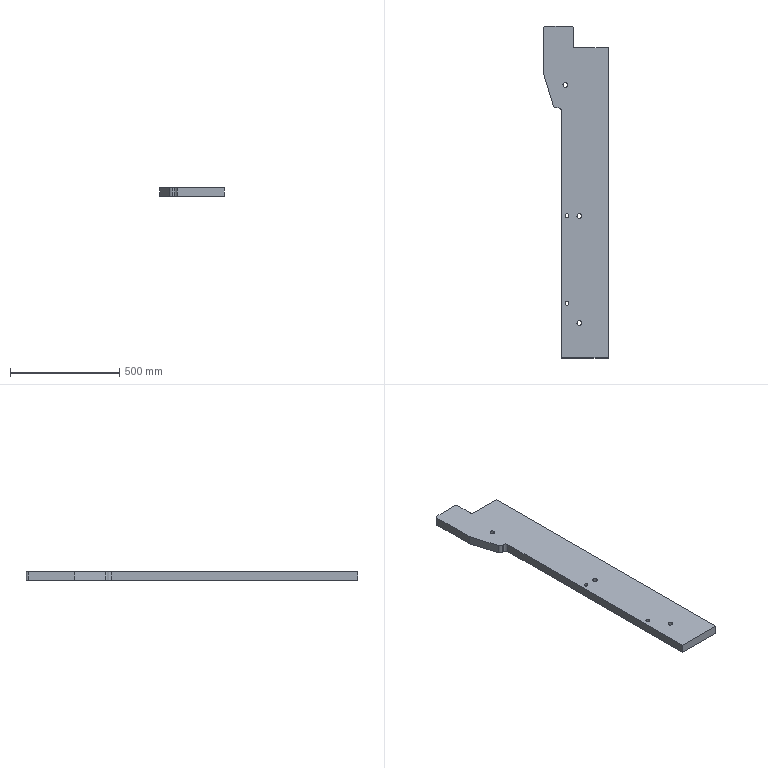Part | SolidWorks | features Fillet 2, 3DProfileFeature 1, Extrusion 1, HoleWzd 1 | 1 solid | 26 faces | box 295.68 x 1520 x 40 mm | volume 13433677 mm3 | cylinder 15 | plane 11 | commonest cylinder face diameters 21 x6 18 x4 20 x3 30 x2
STEP:
#1=CARTESIAN_POINT('',(28.633,1250.,40.));
#2=VERTEX_POINT('',#1);
#3=CARTESIAN_POINT('',(7.633,1250.,40.));
#4=VERTEX_POINT('',#3);
#5=CARTESIAN_POINT('',(18.133,1250.,40.));
#6=DIRECTION('',(0.,0.,-1.));
#7=DIRECTION('',(-1.,0.,0.));
#8=AXIS2_PLACEMENT_3D('',#5,#6,#7);
#9=CIRCLE('',#8,10.5);
#10=EDGE_CURVE('',#2,#4,#9,.T.);
#11=ORIENTED_EDGE('',*,*,#10,.F.);
#12=CARTESIAN_POINT('',(28.633,1250.,0.));
#13=VERTEX_POINT('',#12);
#14=CARTESIAN_POINT('',(28.633,1250.,0.));
#15=DIRECTION('',(0.,0.,-1.));
#16=VECTOR('',#15,1000.);
#17=LINE('',#14,#16);
#18=EDGE_CURVE('',#2,#13,#17,.T.);
#19=ORIENTED_EDGE('',*,*,#18,.T.);
#20=CARTESIAN_POINT('',(7.633,1250.,0.));
#21=VERTEX_POINT('',#20);
#22=CARTESIAN_POINT('',(18.133,1250.,0.));
#23=DIRECTION('',(0.,0.,-1.));
#24=DIRECTION('',(-1.,0.,0.));
#25=AXIS2_PLACEMENT_3D('',#22,#23,#24);
#26=CIRCLE('',#25,10.5);
#27=EDGE_CURVE('',#13,#21,#26,.T.);
#28=ORIENTED_EDGE('',*,*,#27,.T.);
#29=CARTESIAN_POINT('',(7.633,1250.,0.));
#30=DIRECTION('',(0.,0.,-1.));
#31=VECTOR('',#30,1000.);
#32=LINE('',#29,#31);
#33=EDGE_CURVE('',#4,#21,#32,.T.);
#34=ORIENTED_EDGE('',*,*,#33,.F.);
#35=EDGE_LOOP('',(#11,#19,#28,#34));
#36=FACE_OUTER_BOUND('',#35,.T.);
#37=CARTESIAN_POINT('',(18.133,1250.,0.));
#38=DIRECTION('',(0.,0.,-1.));
#39=DIRECTION('',(-1.,0.,0.));
#40=AXIS2_PLACEMENT_3D('',#37,#38,#39);
#41=CYLINDRICAL_SURFACE('',#40,10.5);
#42=ADVANCED_FACE('',(#36),#41,.F.);
#43=CARTESIAN_POINT('',(92.5,650.,40.));
#44=VERTEX_POINT('',#43);
#45=CARTESIAN_POINT('',(71.5,650.,40.));
#46=VERTEX_POINT('',#45);
#47=CARTESIAN_POINT('',(82.,650.,40.));
#48=DIRECTION('',(0.,0.,-1.));
#49=DIRECTION('',(-1.,0.,0.));
#50=AXIS2_PLACEMENT_3D('',#47,#48,#49);
#51=CIRCLE('',#50,10.5);
#52=EDGE_CURVE('',#44,#46,#51,.T.);
#53=ORIENTED_EDGE('',*,*,#52,.F.);
#54=CARTESIAN_POINT('',(92.5,650.,0.));
#55=VERTEX_POINT('',#54);
#56=CARTESIAN_POINT('',(92.5,650.,0.));
#57=DIRECTION('',(0.,0.,-1.));
#58=VECTOR('',#57,1000.);
#59=LINE('',#56,#58);
#60=EDGE_CURVE('',#44,#55,#59,.T.);
#61=ORIENTED_EDGE('',*,*,#60,.T.);
#62=CARTESIAN_POINT('',(71.5,650.,0.));
#63=VERTEX_POINT('',#62);
#64=CARTESIAN_POINT('',(82.,650.,0.));
#65=DIRECTION('',(0.,0.,-1.));
#66=DIRECTION('',(-1.,0.,0.));
#67=AXIS2_PLACEMENT_3D('',#64,#65,#66);
#68=CIRCLE('',#67,10.5);
#69=EDGE_CURVE('',#55,#63,#68,.T.);
#70=ORIENTED_EDGE('',*,*,#69,.T.);
#71=CARTESIAN_POINT('',(71.5,650.,0.));
#72=DIRECTION('',(0.,0.,-1.));
#73=VECTOR('',#72,1000.);
#74=LINE('',#71,#73);
#75=EDGE_CURVE('',#46,#63,#74,.T.);
#76=ORIENTED_EDGE('',*,*,#75,.F.);
#77=EDGE_LOOP('',(#53,#61,#70,#76));
#78=FACE_OUTER_BOUND('',#77,.T.);
#79=CARTESIAN_POINT('',(82.,650.,0.));
#80=DIRECTION('',(0.,0.,-1.));
#81=DIRECTION('',(-1.,0.,0.));
#82=AXIS2_PLACEMENT_3D('',#79,#80,#81);
#83=CYLINDRICAL_SURFACE('',#82,10.5);
#84=ADVANCED_FACE('',(#78),#83,.F.);
#85=CARTESIAN_POINT('',(92.5,160.,40.));
#86=VERTEX_POINT('',#85);
#87=CARTESIAN_POINT('',(71.5,160.,40.));
#88=VERTEX_POINT('',#87);
#89=CARTESIAN_POINT('',(82.,160.,40.));
#90=DIRECTION('',(0.,0.,-1.));
#91=DIRECTION('',(-1.,0.,0.));
#92=AXIS2_PLACEMENT_3D('',#89,#90,#91);
#93=CIRCLE('',#92,10.5);
#94=EDGE_CURVE('',#86,#88,#93,.T.);
#95=ORIENTED_EDGE('',*,*,#94,.F.);
#96=CARTESIAN_POINT('',(92.5,160.,0.));
#97=VERTEX_POINT('',#96);
#98=CARTESIAN_POINT('',(92.5,160.,0.));
#99=DIRECTION('',(0.,0.,-1.));
#100=VECTOR('',#99,1000.);
#101=LINE('',#98,#100);
#102=EDGE_CURVE('',#86,#97,#101,.T.);
#103=ORIENTED_EDGE('',*,*,#102,.T.);
#104=CARTESIAN_POINT('',(71.5,160.,0.));
#105=VERTEX_POINT('',#104);
#106=CARTESIAN_POINT('',(82.,160.,0.));
#107=DIRECTION('',(0.,0.,-1.));
#108=DIRECTION('',(-1.,0.,0.));
#109=AXIS2_PLACEMENT_3D('',#106,#107,#108);
#110=CIRCLE('',#109,10.5);
#111=EDGE_CURVE('',#97,#105,#110,.T.);
#112=ORIENTED_EDGE('',*,*,#111,.T.);
#113=CARTESIAN_POINT('',(71.5,160.,0.));
#114=DIRECTION('',(0.,0.,-1.));
#115=VECTOR('',#114,1000.);
#116=LINE('',#113,#115);
#117=EDGE_CURVE('',#88,#105,#116,.T.);
#118=ORIENTED_EDGE('',*,*,#117,.F.);
#119=EDGE_LOOP('',(#95,#103,#112,#118));
#120=FACE_OUTER_BOUND('',#119,.T.);
#121=CARTESIAN_POINT('',(82.,160.,0.));
#122=DIRECTION('',(0.,0.,-1.));
#123=DIRECTION('',(-1.,0.,0.));
#124=AXIS2_PLACEMENT_3D('',#121,#122,#123);
#125=CYLINDRICAL_SURFACE('',#124,10.5);
#126=ADVANCED_FACE('',(#120),#125,.F.);
#127=CARTESIAN_POINT('',(17.,651.,40.));
#128=VERTEX_POINT('',#127);
#129=CARTESIAN_POINT('',(35.,651.,40.));
#130=VERTEX_POINT('',#129);
#131=CARTESIAN_POINT('',(26.,651.,40.));
#132=DIRECTION('',(0.,0.,1.));
#133=DIRECTION('',(1.,0.,0.));
#134=AXIS2_PLACEMENT_3D('',#131,#132,#133);
#135=CIRCLE('',#134,9.);
#136=EDGE_CURVE('',#128,#130,#135,.T.);
#137=ORIENTED_EDGE('',*,*,#136,.T.);
#138=CARTESIAN_POINT('',(35.,651.,0.));
#139=VERTEX_POINT('',#138);
#140=CARTESIAN_POINT('',(35.,651.,40.));
#141=DIRECTION('',(0.,0.,-1.));
#142=VECTOR('',#141,1000.);
#143=LINE('',#140,#142);
#144=EDGE_CURVE('',#130,#139,#143,.T.);
#145=ORIENTED_EDGE('',*,*,#144,.T.);
#146=CARTESIAN_POINT('',(17.,651.,0.));
#147=VERTEX_POINT('',#146);
#148=CARTESIAN_POINT('',(26.,651.,0.));
#149=DIRECTION('',(0.,0.,1.));
#150=DIRECTION('',(1.,0.,0.));
#151=AXIS2_PLACEMENT_3D('',#148,#149,#150);
#152=CIRCLE('',#151,9.);
#153=EDGE_CURVE('',#147,#139,#152,.T.);
#154=ORIENTED_EDGE('',*,*,#153,.F.);
#155=CARTESIAN_POINT('',(17.,651.,40.));
#156=DIRECTION('',(0.,0.,-1.));
#157=VECTOR('',#156,1000.);
#158=LINE('',#155,#157);
#159=EDGE_CURVE('',#128,#147,#158,.T.);
#160=ORIENTED_EDGE('',*,*,#159,.F.);
#161=EDGE_LOOP('',(#137,#145,#154,#160));
#162=FACE_OUTER_BOUND('',#161,.T.);
#163=CARTESIAN_POINT('',(26.,651.,40.));
#164=DIRECTION('',(0.,0.,-1.));
#165=DIRECTION('',(-1.,0.,0.));
#166=AXIS2_PLACEMENT_3D('',#163,#164,#165);
#167=CYLINDRICAL_SURFACE('',#166,9.);
#168=ADVANCED_FACE('',(#162),#167,.F.);
#169=CARTESIAN_POINT('',(17.,251.,40.));
#170=VERTEX_POINT('',#169);
#171=CARTESIAN_POINT('',(35.,251.,40.));
#172=VERTEX_POINT('',#171);
#173=CARTESIAN_POINT('',(26.,251.,40.));
#174=DIRECTION('',(0.,0.,1.));
#175=DIRECTION('',(1.,0.,0.));
#176=AXIS2_PLACEMENT_3D('',#173,#174,#175);
#177=CIRCLE('',#176,9.);
#178=EDGE_CURVE('',#170,#172,#177,.T.);
#179=ORIENTED_EDGE('',*,*,#178,.T.);
#180=CARTESIAN_POINT('',(35.,251.,0.));
#181=VERTEX_POINT('',#180);
#182=CARTESIAN_POINT('',(35.,251.,40.));
#183=DIRECTION('',(0.,0.,-1.));
#184=VECTOR('',#183,1000.);
#185=LINE('',#182,#184);
#186=EDGE_CURVE('',#172,#181,#185,.T.);
#187=ORIENTED_EDGE('',*,*,#186,.T.);
#188=CARTESIAN_POINT('',(17.,251.,0.));
#189=VERTEX_POINT('',#188);
#190=CARTESIAN_POINT('',(26.,251.,0.));
#191=DIRECTION('',(0.,0.,1.));
#192=DIRECTION('',(1.,0.,0.));
#193=AXIS2_PLACEMENT_3D('',#190,#191,#192);
#194=CIRCLE('',#193,9.);
#195=EDGE_CURVE('',#189,#181,#194,.T.);
#196=ORIENTED_EDGE('',*,*,#195,.F.);
#197=CARTESIAN_POINT('',(17.,251.,40.));
#198=DIRECTION('',(0.,0.,-1.));
#199=VECTOR('',#198,1000.);
#200=LINE('',#197,#199);
#201=EDGE_CURVE('',#170,#189,#200,.T.);
#202=ORIENTED_EDGE('',*,*,#201,.F.);
#203=EDGE_LOOP('',(#179,#187,#196,#202));
#204=FACE_OUTER_BOUND('',#203,.T.);
#205=CARTESIAN_POINT('',(26.,251.,40.));
#206=DIRECTION('',(0.,0.,-1.));
#207=DIRECTION('',(-1.,0.,0.));
#208=AXIS2_PLACEMENT_3D('',#205,#206,#207);
#209=CYLINDRICAL_SURFACE('',#208,9.);
#210=ADVANCED_FACE('',(#204),#209,.F.);
#211=CARTESIAN_POINT('',(18.133,1250.,40.));
#212=DIRECTION('',(0.,0.,-1.));
#213=DIRECTION('',(-1.,0.,0.));
#214=AXIS2_PLACEMENT_3D('',#211,#212,#213);
#215=CIRCLE('',#214,10.5);
#216=EDGE_CURVE('',#4,#2,#215,.T.);
#217=ORIENTED_EDGE('',*,*,#216,.T.);
#218=ORIENTED_EDGE('',*,*,#10,.T.);
#219=EDGE_LOOP('',(#217,#218));
#220=FACE_BOUND('',#219,.T.);
#221=CARTESIAN_POINT('',(82.,650.,40.));
#222=DIRECTION('',(0.,0.,-1.));
#223=DIRECTION('',(-1.,0.,0.));
#224=AXIS2_PLACEMENT_3D('',#221,#222,#223);
#225=CIRCLE('',#224,10.5);
#226=EDGE_CURVE('',#46,#44,#225,.T.);
#227=ORIENTED_EDGE('',*,*,#226,.T.);
#228=ORIENTED_EDGE('',*,*,#52,.T.);
#229=EDGE_LOOP('',(#227,#228));
#230=FACE_BOUND('',#229,.T.);
#231=CARTESIAN_POINT('',(82.,160.,40.));
#232=DIRECTION('',(0.,0.,-1.));
#233=DIRECTION('',(-1.,0.,0.));
#234=AXIS2_PLACEMENT_3D('',#231,#232,#233);
#235=CIRCLE('',#234,10.5);
#236=EDGE_CURVE('',#88,#86,#235,.T.);
#237=ORIENTED_EDGE('',*,*,#236,.T.);
#238=ORIENTED_EDGE('',*,*,#94,.T.);
#239=EDGE_LOOP('',(#237,#238));
#240=FACE_BOUND('',#239,.T.);
#241=CARTESIAN_POINT('',(45.,1520.,40.));
#242=VERTEX_POINT('',#241);
#243=CARTESIAN_POINT('',(-70.68,1520.,40.));
#244=VERTEX_POINT('',#243);
#245=CARTESIAN_POINT('',(55.,1520.,40.));
#246=DIRECTION('',(-1.,0.,0.));
#247=VECTOR('',#246,1000.);
#248=LINE('',#245,#247);
#249=EDGE_CURVE('',#242,#244,#248,.T.);
#250=ORIENTED_EDGE('',*,*,#249,.T.);
#251=CARTESIAN_POINT('',(-80.68,1510.,40.));
#252=VERTEX_POINT('',#251);
#253=CARTESIAN_POINT('',(-70.68,1510.,40.));
#254=DIRECTION('',(0.,0.,1.));
#255=DIRECTION('',(-1.,0.,0.));
#256=AXIS2_PLACEMENT_3D('',#253,#254,#255);
#257=CIRCLE('',#256,10.);
#258=EDGE_CURVE('',#244,#252,#257,.T.);
#259=ORIENTED_EDGE('',*,*,#258,.T.);
#260=CARTESIAN_POINT('',(-80.68,1300.,40.));
#261=VERTEX_POINT('',#260);
#262=CARTESIAN_POINT('',(-80.68,1300.,40.));
#263=DIRECTION('',(0.,-1.,0.));
#264=VECTOR('',#263,1000.);
#265=LINE('',#262,#264);
#266=EDGE_CURVE('',#252,#261,#265,.T.);
#267=ORIENTED_EDGE('',*,*,#266,.T.);
#268=CARTESIAN_POINT('',(-36.957,1156.154,40.));
#269=VERTEX_POINT('',#268);
#270=CARTESIAN_POINT('',(-33.724,1145.516,40.));
#271=DIRECTION('',(0.2908,-0.9568,0.));
#272=VECTOR('',#271,1000.);
#273=LINE('',#270,#272);
#274=EDGE_CURVE('',#261,#269,#273,.T.);
#275=ORIENTED_EDGE('',*,*,#274,.T.);
#276=CARTESIAN_POINT('',(-22.606,1145.516,40.));
#277=VERTEX_POINT('',#276);
#278=CARTESIAN_POINT('',(-22.606,1160.516,40.));
#279=DIRECTION('',(0.,0.,1.));
#280=DIRECTION('',(-1.,0.,0.));
#281=AXIS2_PLACEMENT_3D('',#278,#279,#280);
#282=CIRCLE('',#281,15.);
#283=EDGE_CURVE('',#269,#277,#282,.T.);
#284=ORIENTED_EDGE('',*,*,#283,.T.);
#285=CARTESIAN_POINT('',(-15.,1145.516,40.));
#286=VERTEX_POINT('',#285);
#287=CARTESIAN_POINT('',(-33.724,1145.516,40.));
#288=DIRECTION('',(1.,0.,0.));
#289=VECTOR('',#288,1000.);
#290=LINE('',#287,#289);
#291=EDGE_CURVE('',#277,#286,#290,.T.);
#292=ORIENTED_EDGE('',*,*,#291,.T.);
#293=CARTESIAN_POINT('',(0.,1130.516,40.));
#294=VERTEX_POINT('',#293);
#295=CARTESIAN_POINT('',(-15.,1130.516,40.));
#296=DIRECTION('',(0.,0.,-1.));
#297=DIRECTION('',(-1.,0.,0.));
#298=AXIS2_PLACEMENT_3D('',#295,#296,#297);
#299=CIRCLE('',#298,15.);
#300=EDGE_CURVE('',#286,#294,#299,.T.);
#301=ORIENTED_EDGE('',*,*,#300,.T.);
#302=CARTESIAN_POINT('',(0.,0.,40.));
#303=VERTEX_POINT('',#302);
#304=CARTESIAN_POINT('',(0.,0.,40.));
#305=DIRECTION('',(0.,-1.,0.));
#306=VECTOR('',#305,1000.);
#307=LINE('',#304,#306);
#308=EDGE_CURVE('',#294,#303,#307,.T.);
#309=ORIENTED_EDGE('',*,*,#308,.T.);
#310=CARTESIAN_POINT('',(215.,0.,40.));
#311=VERTEX_POINT('',#310);
#312=CARTESIAN_POINT('',(215.,0.,40.));
#313=DIRECTION('',(1.,0.,0.));
#314=VECTOR('',#313,1000.);
#315=LINE('',#312,#314);
#316=EDGE_CURVE('',#303,#311,#315,.T.);
#317=ORIENTED_EDGE('',*,*,#316,.T.);
#318=CARTESIAN_POINT('',(215.,1420.,40.));
#319=VERTEX_POINT('',#318);
#320=CARTESIAN_POINT('',(215.,1420.,40.));
#321=DIRECTION('',(0.,1.,0.));
#322=VECTOR('',#321,1000.);
#323=LINE('',#320,#322);
#324=EDGE_CURVE('',#311,#319,#323,.T.);
#325=ORIENTED_EDGE('',*,*,#324,.T.);
#326=CARTESIAN_POINT('',(65.,1420.,40.));
#327=VERTEX_POINT('',#326);
#328=CARTESIAN_POINT('',(215.,1420.,40.));
#329=DIRECTION('',(-1.,0.,0.));
#330=VECTOR('',#329,1000.);
#331=LINE('',#328,#330);
#332=EDGE_CURVE('',#319,#327,#331,.T.);
#333=ORIENTED_EDGE('',*,*,#332,.T.);
#334=CARTESIAN_POINT('',(55.,1430.,40.));
#335=VERTEX_POINT('',#334);
#336=CARTESIAN_POINT('',(65.,1430.,40.));
#337=DIRECTION('',(0.,0.,-1.));
#338=DIRECTION('',(-1.,0.,0.));
#339=AXIS2_PLACEMENT_3D('',#336,#337,#338);
#340=CIRCLE('',#339,10.);
#341=EDGE_CURVE('',#327,#335,#340,.T.);
#342=ORIENTED_EDGE('',*,*,#341,.T.);
#343=CARTESIAN_POINT('',(55.,1510.,40.));
#344=VERTEX_POINT('',#343);
#345=CARTESIAN_POINT('',(55.,1420.,40.));
#346=DIRECTION('',(0.,1.,0.));
#347=VECTOR('',#346,1000.);
#348=LINE('',#345,#347);
#349=EDGE_CURVE('',#335,#344,#348,.T.);
#350=ORIENTED_EDGE('',*,*,#349,.T.);
#351=CARTESIAN_POINT('',(45.,1510.,40.));
#352=DIRECTION('',(0.,0.,1.));
#353=DIRECTION('',(-1.,0.,0.));
#354=AXIS2_PLACEMENT_3D('',#351,#352,#353);
#355=CIRCLE('',#354,10.);
#356=EDGE_CURVE('',#344,#242,#355,.T.);
#357=ORIENTED_EDGE('',*,*,#356,.T.);
#358=EDGE_LOOP('',(#250,#259,#267,#275,#284,#292,#301,#309,#317,#325,#333,#342,#350,#357));
#359=FACE_OUTER_BOUND('',#358,.T.);
#360=ORIENTED_EDGE('',*,*,#178,.F.);
#361=CARTESIAN_POINT('',(26.,251.,40.));
#362=DIRECTION('',(0.,0.,1.));
#363=DIRECTION('',(1.,0.,0.));
#364=AXIS2_PLACEMENT_3D('',#361,#362,#363);
#365=CIRCLE('',#364,9.);
#366=EDGE_CURVE('',#172,#170,#365,.T.);
#367=ORIENTED_EDGE('',*,*,#366,.F.);
#368=EDGE_LOOP('',(#360,#367));
#369=FACE_BOUND('',#368,.T.);
#370=ORIENTED_EDGE('',*,*,#136,.F.);
#371=CARTESIAN_POINT('',(26.,651.,40.));
#372=DIRECTION('',(0.,0.,1.));
#373=DIRECTION('',(1.,0.,0.));
#374=AXIS2_PLACEMENT_3D('',#371,#372,#373);
#375=CIRCLE('',#374,9.);
#376=EDGE_CURVE('',#130,#128,#375,.T.);
#377=ORIENTED_EDGE('',*,*,#376,.F.);
#378=EDGE_LOOP('',(#370,#377));
#379=FACE_BOUND('',#378,.T.);
#380=CARTESIAN_POINT('',(0.,0.,40.));
#381=DIRECTION('',(0.,0.,-1.));
#382=DIRECTION('',(-1.,0.,0.));
#383=AXIS2_PLACEMENT_3D('',#380,#381,#382);
#384=PLANE('',#383);
#385=ADVANCED_FACE('',(#220,#230,#240,#359,#369,#379),#384,.F.);
#386=CARTESIAN_POINT('',(18.133,1250.,0.));
#387=DIRECTION('',(0.,0.,-1.));
#388=DIRECTION('',(-1.,0.,0.));
#389=AXIS2_PLACEMENT_3D('',#386,#387,#388);
#390=CIRCLE('',#389,10.5);
#391=EDGE_CURVE('',#21,#13,#390,.T.);
#392=ORIENTED_EDGE('',*,*,#391,.F.);
#393=ORIENTED_EDGE('',*,*,#27,.F.);
#394=EDGE_LOOP('',(#392,#393));
#395=FACE_BOUND('',#394,.T.);
#396=CARTESIAN_POINT('',(82.,650.,0.));
#397=DIRECTION('',(0.,0.,-1.));
#398=DIRECTION('',(-1.,0.,0.));
#399=AXIS2_PLACEMENT_3D('',#396,#397,#398);
#400=CIRCLE('',#399,10.5);
#401=EDGE_CURVE('',#63,#55,#400,.T.);
#402=ORIENTED_EDGE('',*,*,#401,.F.);
#403=ORIENTED_EDGE('',*,*,#69,.F.);
#404=EDGE_LOOP('',(#402,#403));
#405=FACE_BOUND('',#404,.T.);
#406=CARTESIAN_POINT('',(82.,160.,0.));
#407=DIRECTION('',(0.,0.,-1.));
#408=DIRECTION('',(-1.,0.,0.));
#409=AXIS2_PLACEMENT_3D('',#406,#407,#408);
#410=CIRCLE('',#409,10.5);
#411=EDGE_CURVE('',#105,#97,#410,.T.);
#412=ORIENTED_EDGE('',*,*,#411,.F.);
#413=ORIENTED_EDGE('',*,*,#111,.F.);
#414=EDGE_LOOP('',(#412,#413));
#415=FACE_BOUND('',#414,.T.);
#416=ORIENTED_EDGE('',*,*,#195,.T.);
#417=CARTESIAN_POINT('',(26.,251.,0.));
#418=DIRECTION('',(0.,0.,1.));
#419=DIRECTION('',(1.,0.,0.));
#420=AXIS2_PLACEMENT_3D('',#417,#418,#419);
#421=CIRCLE('',#420,9.);
#422=EDGE_CURVE('',#181,#189,#421,.T.);
#423=ORIENTED_EDGE('',*,*,#422,.T.);
#424=EDGE_LOOP('',(#416,#423));
#425=FACE_BOUND('',#424,.T.);
#426=CARTESIAN_POINT('',(-80.68,1510.,0.));
#427=VERTEX_POINT('',#426);
#428=CARTESIAN_POINT('',(-80.68,1300.,0.));
#429=VERTEX_POINT('',#428);
#430=CARTESIAN_POINT('',(-80.68,1300.,0.));
#431=DIRECTION('',(0.,-1.,0.));
#432=VECTOR('',#431,1000.);
#433=LINE('',#430,#432);
#434=EDGE_CURVE('',#427,#429,#433,.T.);
#435=ORIENTED_EDGE('',*,*,#434,.F.);
#436=CARTESIAN_POINT('',(-70.68,1520.,0.));
#437=VERTEX_POINT('',#436);
#438=CARTESIAN_POINT('',(-70.68,1510.,0.));
#439=DIRECTION('',(0.,0.,-1.));
#440=DIRECTION('',(-1.,0.,0.));
#441=AXIS2_PLACEMENT_3D('',#438,#439,#440);
#442=CIRCLE('',#441,10.);
#443=EDGE_CURVE('',#427,#437,#442,.T.);
#444=ORIENTED_EDGE('',*,*,#443,.T.);
#445=CARTESIAN_POINT('',(45.,1520.,0.));
#446=VERTEX_POINT('',#445);
#447=CARTESIAN_POINT('',(55.,1520.,0.));
#448=DIRECTION('',(-1.,0.,0.));
#449=VECTOR('',#448,1000.);
#450=LINE('',#447,#449);
#451=EDGE_CURVE('',#446,#437,#450,.T.);
#452=ORIENTED_EDGE('',*,*,#451,.F.);
#453=CARTESIAN_POINT('',(55.,1510.,0.));
#454=VERTEX_POINT('',#453);
#455=CARTESIAN_POINT('',(45.,1510.,0.));
#456=DIRECTION('',(0.,0.,-1.));
#457=DIRECTION('',(-1.,0.,0.));
#458=AXIS2_PLACEMENT_3D('',#455,#456,#457);
#459=CIRCLE('',#458,10.);
#460=EDGE_CURVE('',#446,#454,#459,.T.);
#461=ORIENTED_EDGE('',*,*,#460,.T.);
#462=CARTESIAN_POINT('',(55.,1430.,0.));
#463=VERTEX_POINT('',#462);
#464=CARTESIAN_POINT('',(55.,1420.,0.));
#465=DIRECTION('',(0.,1.,0.));
#466=VECTOR('',#465,1000.);
#467=LINE('',#464,#466);
#468=EDGE_CURVE('',#463,#454,#467,.T.);
#469=ORIENTED_EDGE('',*,*,#468,.F.);
#470=CARTESIAN_POINT('',(65.,1420.,0.));
#471=VERTEX_POINT('',#470);
#472=CARTESIAN_POINT('',(65.,1430.,0.));
#473=DIRECTION('',(0.,0.,1.));
#474=DIRECTION('',(-1.,0.,0.));
#475=AXIS2_PLACEMENT_3D('',#472,#473,#474);
#476=CIRCLE('',#475,10.);
#477=EDGE_CURVE('',#463,#471,#476,.T.);
#478=ORIENTED_EDGE('',*,*,#477,.T.);
#479=CARTESIAN_POINT('',(215.,1420.,0.));
#480=VERTEX_POINT('',#479);
#481=CARTESIAN_POINT('',(215.,1420.,0.));
#482=DIRECTION('',(-1.,0.,0.));
#483=VECTOR('',#482,1000.);
#484=LINE('',#481,#483);
#485=EDGE_CURVE('',#480,#471,#484,.T.);
#486=ORIENTED_EDGE('',*,*,#485,.F.);
#487=CARTESIAN_POINT('',(215.,0.,0.));
#488=VERTEX_POINT('',#487);
#489=CARTESIAN_POINT('',(215.,1420.,0.));
#490=DIRECTION('',(0.,1.,0.));
#491=VECTOR('',#490,1000.);
#492=LINE('',#489,#491);
#493=EDGE_CURVE('',#488,#480,#492,.T.);
#494=ORIENTED_EDGE('',*,*,#493,.F.);
#495=CARTESIAN_POINT('',(0.,0.,0.));
#496=VERTEX_POINT('',#495);
#497=CARTESIAN_POINT('',(215.,0.,0.));
#498=DIRECTION('',(1.,0.,0.));
#499=VECTOR('',#498,1000.);
#500=LINE('',#497,#499);
#501=EDGE_CURVE('',#496,#488,#500,.T.);
#502=ORIENTED_EDGE('',*,*,#501,.F.);
#503=CARTESIAN_POINT('',(0.,1130.516,0.));
#504=VERTEX_POINT('',#503);
#505=CARTESIAN_POINT('',(0.,0.,0.));
#506=DIRECTION('',(0.,-1.,0.));
#507=VECTOR('',#506,1000.);
#508=LINE('',#505,#507);
#509=EDGE_CURVE('',#504,#496,#508,.T.);
#510=ORIENTED_EDGE('',*,*,#509,.F.);
#511=CARTESIAN_POINT('',(-15.,1145.516,0.));
#512=VERTEX_POINT('',#511);
#513=CARTESIAN_POINT('',(-15.,1130.516,0.));
#514=DIRECTION('',(0.,0.,1.));
#515=DIRECTION('',(-1.,0.,0.));
#516=AXIS2_PLACEMENT_3D('',#513,#514,#515);
#517=CIRCLE('',#516,15.);
#518=EDGE_CURVE('',#504,#512,#517,.T.);
#519=ORIENTED_EDGE('',*,*,#518,.T.);
#520=CARTESIAN_POINT('',(-22.606,1145.516,0.));
#521=VERTEX_POINT('',#520);
#522=CARTESIAN_POINT('',(-33.724,1145.516,0.));
#523=DIRECTION('',(1.,0.,0.));
#524=VECTOR('',#523,1000.);
#525=LINE('',#522,#524);
#526=EDGE_CURVE('',#521,#512,#525,.T.);
#527=ORIENTED_EDGE('',*,*,#526,.F.);
#528=CARTESIAN_POINT('',(-36.957,1156.154,0.));
#529=VERTEX_POINT('',#528);
#530=CARTESIAN_POINT('',(-22.606,1160.516,0.));
#531=DIRECTION('',(0.,0.,-1.));
#532=DIRECTION('',(-1.,0.,0.));
#533=AXIS2_PLACEMENT_3D('',#530,#531,#532);
#534=CIRCLE('',#533,15.);
#535=EDGE_CURVE('',#521,#529,#534,.T.);
#536=ORIENTED_EDGE('',*,*,#535,.T.);
#537=CARTESIAN_POINT('',(-33.724,1145.516,0.));
#538=DIRECTION('',(0.2908,-0.9568,0.));
#539=VECTOR('',#538,1000.);
#540=LINE('',#537,#539);
#541=EDGE_CURVE('',#429,#529,#540,.T.);
#542=ORIENTED_EDGE('',*,*,#541,.F.);
#543=EDGE_LOOP('',(#435,#444,#452,#461,#469,#478,#486,#494,#502,#510,#519,#527,#536,#542));
#544=FACE_OUTER_BOUND('',#543,.T.);
#545=ORIENTED_EDGE('',*,*,#153,.T.);
#546=CARTESIAN_POINT('',(26.,651.,0.));
#547=DIRECTION('',(0.,0.,1.));
#548=DIRECTION('',(1.,0.,0.));
#549=AXIS2_PLACEMENT_3D('',#546,#547,#548);
#550=CIRCLE('',#549,9.);
#551=EDGE_CURVE('',#139,#147,#550,.T.);
#552=ORIENTED_EDGE('',*,*,#551,.T.);
#553=EDGE_LOOP('',(#545,#552));
#554=FACE_BOUND('',#553,.T.);
#555=CARTESIAN_POINT('',(0.,0.,0.));
#556=DIRECTION('',(0.,0.,-1.));
#557=DIRECTION('',(-1.,0.,0.));
#558=AXIS2_PLACEMENT_3D('',#555,#556,#557);
#559=PLANE('',#558);
#560=ADVANCED_FACE('',(#395,#405,#415,#425,#544,#554),#559,.T.);
#561=ORIENTED_EDGE('',*,*,#501,.T.);
#562=CARTESIAN_POINT('',(215.,0.,40.));
#563=DIRECTION('',(0.,0.,-1.));
#564=VECTOR('',#563,1000.);
#565=LINE('',#562,#564);
#566=EDGE_CURVE('',#311,#488,#565,.T.);
#567=ORIENTED_EDGE('',*,*,#566,.F.);
#568=ORIENTED_EDGE('',*,*,#316,.F.);
#569=CARTESIAN_POINT('',(0.,0.,40.));
#570=DIRECTION('',(0.,0.,-1.));
#571=VECTOR('',#570,1000.);
#572=LINE('',#569,#571);
#573=EDGE_CURVE('',#303,#496,#572,.T.);
#574=ORIENTED_EDGE('',*,*,#573,.T.);
#575=EDGE_LOOP('',(#561,#567,#568,#574));
#576=FACE_OUTER_BOUND('',#575,.T.);
#577=CARTESIAN_POINT('',(215.,0.,40.));
#578=DIRECTION('',(0.,1.,0.));
#579=DIRECTION('',(-1.,0.,0.));
#580=AXIS2_PLACEMENT_3D('',#577,#578,#579);
#581=PLANE('',#580);
#582=ADVANCED_FACE('',(#576),#581,.F.);
#583=ORIENTED_EDGE('',*,*,#493,.T.);
#584=CARTESIAN_POINT('',(215.,1420.,40.));
#585=DIRECTION('',(0.,0.,-1.));
#586=VECTOR('',#585,1000.);
#587=LINE('',#584,#586);
#588=EDGE_CURVE('',#319,#480,#587,.T.);
#589=ORIENTED_EDGE('',*,*,#588,.F.);
#590=ORIENTED_EDGE('',*,*,#324,.F.);
#591=ORIENTED_EDGE('',*,*,#566,.T.);
#592=EDGE_LOOP('',(#583,#589,#590,#591));
#593=FACE_OUTER_BOUND('',#592,.T.);
#594=CARTESIAN_POINT('',(215.,1420.,40.));
#595=DIRECTION('',(-1.,0.,0.));
#596=DIRECTION('',(0.,-1.,0.));
#597=AXIS2_PLACEMENT_3D('',#594,#595,#596);
#598=PLANE('',#597);
#599=ADVANCED_FACE('',(#593),#598,.F.);
#600=ORIENTED_EDGE('',*,*,#485,.T.);
#601=CARTESIAN_POINT('',(65.,1420.,40.));
#602=DIRECTION('',(0.,0.,1.));
#603=VECTOR('',#602,1000.);
#604=LINE('',#601,#603);
#605=EDGE_CURVE('',#471,#327,#604,.T.);
#606=ORIENTED_EDGE('',*,*,#605,.T.);
#607=ORIENTED_EDGE('',*,*,#332,.F.);
#608=ORIENTED_EDGE('',*,*,#588,.T.);
#609=EDGE_LOOP('',(#600,#606,#607,#608));
#610=FACE_OUTER_BOUND('',#609,.T.);
#611=CARTESIAN_POINT('',(215.,1420.,40.));
#612=DIRECTION('',(0.,-1.,0.));
#613=DIRECTION('',(0.,0.,-1.));
#614=AXIS2_PLACEMENT_3D('',#611,#612,#613);
#615=PLANE('',#614);
#616=ADVANCED_FACE('',(#610),#615,.F.);
#617=ORIENTED_EDGE('',*,*,#468,.T.);
#618=CARTESIAN_POINT('',(55.,1510.,40.));
#619=DIRECTION('',(0.,0.,1.));
#620=VECTOR('',#619,1000.);
#621=LINE('',#618,#620);
#622=EDGE_CURVE('',#454,#344,#621,.T.);
#623=ORIENTED_EDGE('',*,*,#622,.T.);
#624=ORIENTED_EDGE('',*,*,#349,.F.);
#625=CARTESIAN_POINT('',(55.,1430.,0.));
#626=DIRECTION('',(0.,0.,-1.));
#627=VECTOR('',#626,1000.);
#628=LINE('',#625,#627);
#629=EDGE_CURVE('',#335,#463,#628,.T.);
#630=ORIENTED_EDGE('',*,*,#629,.T.);
#631=EDGE_LOOP('',(#617,#623,#624,#630));
#632=FACE_OUTER_BOUND('',#631,.T.);
#633=CARTESIAN_POINT('',(55.,1420.,40.));
#634=DIRECTION('',(-1.,0.,0.));
#635=DIRECTION('',(0.,0.,1.));
#636=AXIS2_PLACEMENT_3D('',#633,#634,#635);
#637=PLANE('',#636);
#638=ADVANCED_FACE('',(#632),#637,.F.);
#639=ORIENTED_EDGE('',*,*,#451,.T.);
#640=CARTESIAN_POINT('',(-70.68,1520.,40.));
#641=DIRECTION('',(0.,0.,1.));
#642=VECTOR('',#641,1000.);
#643=LINE('',#640,#642);
#644=EDGE_CURVE('',#437,#244,#643,.T.);
#645=ORIENTED_EDGE('',*,*,#644,.T.);
#646=ORIENTED_EDGE('',*,*,#249,.F.);
#647=CARTESIAN_POINT('',(45.,1520.,40.));
#648=DIRECTION('',(0.,0.,-1.));
#649=VECTOR('',#648,1000.);
#650=LINE('',#647,#649);
#651=EDGE_CURVE('',#242,#446,#650,.T.);
#652=ORIENTED_EDGE('',*,*,#651,.T.);
#653=EDGE_LOOP('',(#639,#645,#646,#652));
#654=FACE_OUTER_BOUND('',#653,.T.);
#655=CARTESIAN_POINT('',(55.,1520.,40.));
#656=DIRECTION('',(0.,-1.,0.));
#657=DIRECTION('',(0.,0.,-1.));
#658=AXIS2_PLACEMENT_3D('',#655,#656,#657);
#659=PLANE('',#658);
#660=ADVANCED_FACE('',(#654),#659,.F.);
#661=ORIENTED_EDGE('',*,*,#266,.F.);
#662=CARTESIAN_POINT('',(-80.68,1510.,40.));
#663=DIRECTION('',(0.,0.,-1.));
#664=VECTOR('',#663,1000.);
#665=LINE('',#662,#664);
#666=EDGE_CURVE('',#252,#427,#665,.T.);
#667=ORIENTED_EDGE('',*,*,#666,.T.);
#668=ORIENTED_EDGE('',*,*,#434,.T.);
#669=CARTESIAN_POINT('',(-80.68,1300.,40.));
#670=DIRECTION('',(0.,0.,-1.));
#671=VECTOR('',#670,1000.);
#672=LINE('',#669,#671);
#673=EDGE_CURVE('',#261,#429,#672,.T.);
#674=ORIENTED_EDGE('',*,*,#673,.F.);
#675=EDGE_LOOP('',(#661,#667,#668,#674));
#676=FACE_OUTER_BOUND('',#675,.T.);
#677=CARTESIAN_POINT('',(-80.68,1300.,40.));
#678=DIRECTION('',(1.,0.,0.));
#679=DIRECTION('',(0.,1.,0.));
#680=AXIS2_PLACEMENT_3D('',#677,#678,#679);
#681=PLANE('',#680);
#682=ADVANCED_FACE('',(#676),#681,.F.);
#683=ORIENTED_EDGE('',*,*,#541,.T.);
#684=CARTESIAN_POINT('',(-36.957,1156.154,40.));
#685=DIRECTION('',(0.,0.,1.));
#686=VECTOR('',#685,1000.);
#687=LINE('',#684,#686);
#688=EDGE_CURVE('',#529,#269,#687,.T.);
#689=ORIENTED_EDGE('',*,*,#688,.T.);
#690=ORIENTED_EDGE('',*,*,#274,.F.);
#691=ORIENTED_EDGE('',*,*,#673,.T.);
#692=EDGE_LOOP('',(#683,#689,#690,#691));
#693=FACE_OUTER_BOUND('',#692,.T.);
#694=CARTESIAN_POINT('',(-33.724,1145.516,40.));
#695=DIRECTION('',(0.9568,0.2908,0.));
#696=DIRECTION('',(-0.2908,0.9568,0.));
#697=AXIS2_PLACEMENT_3D('',#694,#695,#696);
#698=PLANE('',#697);
#699=ADVANCED_FACE('',(#693),#698,.F.);
#700=ORIENTED_EDGE('',*,*,#526,.T.);
#701=CARTESIAN_POINT('',(-15.,1145.516,40.));
#702=DIRECTION('',(0.,0.,1.));
#703=VECTOR('',#702,1000.);
#704=LINE('',#701,#703);
#705=EDGE_CURVE('',#512,#286,#704,.T.);
#706=ORIENTED_EDGE('',*,*,#705,.T.);
#707=ORIENTED_EDGE('',*,*,#291,.F.);
#708=CARTESIAN_POINT('',(-22.606,1145.516,40.));
#709=DIRECTION('',(0.,0.,-1.));
#710=VECTOR('',#709,1000.);
#711=LINE('',#708,#710);
#712=EDGE_CURVE('',#277,#521,#711,.T.);
#713=ORIENTED_EDGE('',*,*,#712,.T.);
#714=EDGE_LOOP('',(#700,#706,#707,#713));
#715=FACE_OUTER_BOUND('',#714,.T.);
#716=CARTESIAN_POINT('',(-33.724,1145.516,40.));
#717=DIRECTION('',(0.,1.,0.));
#718=DIRECTION('',(0.,0.,1.));
#719=AXIS2_PLACEMENT_3D('',#716,#717,#718);
#720=PLANE('',#719);
#721=ADVANCED_FACE('',(#715),#720,.F.);
#722=ORIENTED_EDGE('',*,*,#308,.F.);
#723=CARTESIAN_POINT('',(0.,1130.516,0.));
#724=DIRECTION('',(0.,0.,-1.));
#725=VECTOR('',#724,1000.);
#726=LINE('',#723,#725);
#727=EDGE_CURVE('',#294,#504,#726,.T.);
#728=ORIENTED_EDGE('',*,*,#727,.T.);
#729=ORIENTED_EDGE('',*,*,#509,.T.);
#730=ORIENTED_EDGE('',*,*,#573,.F.);
#731=EDGE_LOOP('',(#722,#728,#729,#730));
#732=FACE_OUTER_BOUND('',#731,.T.);
#733=CARTESIAN_POINT('',(0.,0.,40.));
#734=DIRECTION('',(1.,0.,0.));
#735=DIRECTION('',(0.,0.,-1.));
#736=AXIS2_PLACEMENT_3D('',#733,#734,#735);
#737=PLANE('',#736);
#738=ADVANCED_FACE('',(#732),#737,.F.);
#739=ORIENTED_EDGE('',*,*,#186,.F.);
#740=ORIENTED_EDGE('',*,*,#366,.T.);
#741=ORIENTED_EDGE('',*,*,#201,.T.);
#742=ORIENTED_EDGE('',*,*,#422,.F.);
#743=EDGE_LOOP('',(#739,#740,#741,#742));
#744=FACE_OUTER_BOUND('',#743,.T.);
#745=CARTESIAN_POINT('',(26.,251.,40.));
#746=DIRECTION('',(0.,0.,-1.));
#747=DIRECTION('',(-1.,0.,0.));
#748=AXIS2_PLACEMENT_3D('',#745,#746,#747);
#749=CYLINDRICAL_SURFACE('',#748,9.);
#750=ADVANCED_FACE('',(#744),#749,.F.);
#751=ORIENTED_EDGE('',*,*,#144,.F.);
#752=ORIENTED_EDGE('',*,*,#376,.T.);
#753=ORIENTED_EDGE('',*,*,#159,.T.);
#754=ORIENTED_EDGE('',*,*,#551,.F.);
#755=EDGE_LOOP('',(#751,#752,#753,#754));
#756=FACE_OUTER_BOUND('',#755,.T.);
#757=CARTESIAN_POINT('',(26.,651.,40.));
#758=DIRECTION('',(0.,0.,-1.));
#759=DIRECTION('',(-1.,0.,0.));
#760=AXIS2_PLACEMENT_3D('',#757,#758,#759);
#761=CYLINDRICAL_SURFACE('',#760,9.);
#762=ADVANCED_FACE('',(#756),#761,.F.);
#763=ORIENTED_EDGE('',*,*,#102,.F.);
#764=ORIENTED_EDGE('',*,*,#236,.F.);
#765=ORIENTED_EDGE('',*,*,#117,.T.);
#766=ORIENTED_EDGE('',*,*,#411,.T.);
#767=EDGE_LOOP('',(#763,#764,#765,#766));
#768=FACE_OUTER_BOUND('',#767,.T.);
#769=CARTESIAN_POINT('',(82.,160.,0.));
#770=DIRECTION('',(0.,0.,-1.));
#771=DIRECTION('',(-1.,0.,0.));
#772=AXIS2_PLACEMENT_3D('',#769,#770,#771);
#773=CYLINDRICAL_SURFACE('',#772,10.5);
#774=ADVANCED_FACE('',(#768),#773,.F.);
#775=ORIENTED_EDGE('',*,*,#60,.F.);
#776=ORIENTED_EDGE('',*,*,#226,.F.);
#777=ORIENTED_EDGE('',*,*,#75,.T.);
#778=ORIENTED_EDGE('',*,*,#401,.T.);
#779=EDGE_LOOP('',(#775,#776,#777,#778));
#780=FACE_OUTER_BOUND('',#779,.T.);
#781=CARTESIAN_POINT('',(82.,650.,0.));
#782=DIRECTION('',(0.,0.,-1.));
#783=DIRECTION('',(-1.,0.,0.));
#784=AXIS2_PLACEMENT_3D('',#781,#782,#783);
#785=CYLINDRICAL_SURFACE('',#784,10.5);
#786=ADVANCED_FACE('',(#780),#785,.F.);
#787=ORIENTED_EDGE('',*,*,#18,.F.);
#788=ORIENTED_EDGE('',*,*,#216,.F.);
#789=ORIENTED_EDGE('',*,*,#33,.T.);
#790=ORIENTED_EDGE('',*,*,#391,.T.);
#791=EDGE_LOOP('',(#787,#788,#789,#790));
#792=FACE_OUTER_BOUND('',#791,.T.);
#793=CARTESIAN_POINT('',(18.133,1250.,0.));
#794=DIRECTION('',(0.,0.,-1.));
#795=DIRECTION('',(-1.,0.,0.));
#796=AXIS2_PLACEMENT_3D('',#793,#794,#795);
#797=CYLINDRICAL_SURFACE('',#796,10.5);
#798=ADVANCED_FACE('',(#792),#797,.F.);
#799=ORIENTED_EDGE('',*,*,#300,.F.);
#800=ORIENTED_EDGE('',*,*,#705,.F.);
#801=ORIENTED_EDGE('',*,*,#518,.F.);
#802=ORIENTED_EDGE('',*,*,#727,.F.);
#803=EDGE_LOOP('',(#799,#800,#801,#802));
#804=FACE_OUTER_BOUND('',#803,.T.);
#805=CARTESIAN_POINT('',(-15.,1130.516,40.));
#806=DIRECTION('',(0.,0.,1.));
#807=DIRECTION('',(1.,0.,0.));
#808=AXIS2_PLACEMENT_3D('',#805,#806,#807);
#809=CYLINDRICAL_SURFACE('',#808,15.);
#810=ADVANCED_FACE('',(#804),#809,.F.);
#811=ORIENTED_EDGE('',*,*,#283,.F.);
#812=ORIENTED_EDGE('',*,*,#688,.F.);
#813=ORIENTED_EDGE('',*,*,#535,.F.);
#814=ORIENTED_EDGE('',*,*,#712,.F.);
#815=EDGE_LOOP('',(#811,#812,#813,#814));
#816=FACE_OUTER_BOUND('',#815,.T.);
#817=CARTESIAN_POINT('',(-22.606,1160.516,40.));
#818=DIRECTION('',(0.,0.,-1.));
#819=DIRECTION('',(-1.,0.,0.));
#820=AXIS2_PLACEMENT_3D('',#817,#818,#819);
#821=CYLINDRICAL_SURFACE('',#820,15.);
#822=ADVANCED_FACE('',(#816),#821,.T.);
#823=ORIENTED_EDGE('',*,*,#258,.F.);
#824=ORIENTED_EDGE('',*,*,#644,.F.);
#825=ORIENTED_EDGE('',*,*,#443,.F.);
#826=ORIENTED_EDGE('',*,*,#666,.F.);
#827=EDGE_LOOP('',(#823,#824,#825,#826));
#828=FACE_OUTER_BOUND('',#827,.T.);
#829=CARTESIAN_POINT('',(-70.68,1510.,40.));
#830=DIRECTION('',(0.,0.,-1.));
#831=DIRECTION('',(-1.,0.,0.));
#832=AXIS2_PLACEMENT_3D('',#829,#830,#831);
#833=CYLINDRICAL_SURFACE('',#832,10.);
#834=ADVANCED_FACE('',(#828),#833,.T.);
#835=ORIENTED_EDGE('',*,*,#356,.F.);
#836=ORIENTED_EDGE('',*,*,#622,.F.);
#837=ORIENTED_EDGE('',*,*,#460,.F.);
#838=ORIENTED_EDGE('',*,*,#651,.F.);
#839=EDGE_LOOP('',(#835,#836,#837,#838));
#840=FACE_OUTER_BOUND('',#839,.T.);
#841=CARTESIAN_POINT('',(45.,1510.,40.));
#842=DIRECTION('',(0.,0.,-1.));
#843=DIRECTION('',(-1.,0.,0.));
#844=AXIS2_PLACEMENT_3D('',#841,#842,#843);
#845=CYLINDRICAL_SURFACE('',#844,10.);
#846=ADVANCED_FACE('',(#840),#845,.T.);
#847=ORIENTED_EDGE('',*,*,#341,.F.);
#848=ORIENTED_EDGE('',*,*,#605,.F.);
#849=ORIENTED_EDGE('',*,*,#477,.F.);
#850=ORIENTED_EDGE('',*,*,#629,.F.);
#851=EDGE_LOOP('',(#847,#848,#849,#850));
#852=FACE_OUTER_BOUND('',#851,.T.);
#853=CARTESIAN_POINT('',(65.,1430.,40.));
#854=DIRECTION('',(0.,0.,1.));
#855=DIRECTION('',(1.,0.,0.));
#856=AXIS2_PLACEMENT_3D('',#853,#854,#855);
#857=CYLINDRICAL_SURFACE('',#856,10.);
#858=ADVANCED_FACE('',(#852),#857,.F.);
#859=CLOSED_SHELL('',(#42,#84,#126,#168,#210,#385,#560,#582,#599,#616,#638,#660,#682,#699,#721,#738,#750,#762,#774,#786,#798,#810,#822,#834,#846,#858));
#860=MANIFOLD_SOLID_BREP('',#859);
#861=CARTESIAN_POINT('',(0.,0.,0.));
#862=DIRECTION('',(0.,0.,1.));
#863=DIRECTION('',(1.,0.,0.));
#864=AXIS2_PLACEMENT_3D('',#861,#862,#863);
#865=(LENGTH_UNIT()NAMED_UNIT(*)SI_UNIT(.MILLI.,.METRE.));
#866=UNCERTAINTY_MEASURE_WITH_UNIT(LENGTH_MEASURE(0.00001),#865,'','');
#867=(NAMED_UNIT(*)PLANE_ANGLE_UNIT()SI_UNIT($,.RADIAN.));
#868=(NAMED_UNIT(*)SI_UNIT($,.STERADIAN.)SOLID_ANGLE_UNIT());
#869=(GEOMETRIC_REPRESENTATION_CONTEXT(3)GLOBAL_UNCERTAINTY_ASSIGNED_CONTEXT((#866))GLOBAL_UNIT_ASSIGNED_CONTEXT((#865,#867,#868))REPRESENTATION_CONTEXT('',''));
#870=ADVANCED_BREP_SHAPE_REPRESENTATION('',(#860,#864),#869);